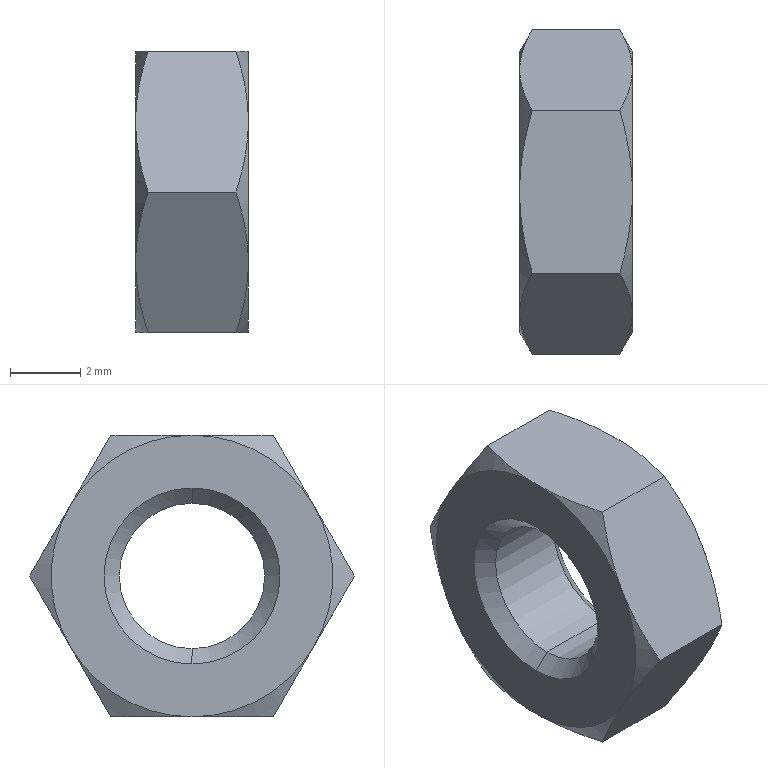Part | SolidWorks | features RefAxis 3, RevCut 2, 3DProfileFeature 1, Extrusion 1 | 1 solid | 26 faces | box 3.2 x 9.238 x 8 mm | volume 130.688 mm3 | cone 16 | plane 8 | cylinder 2 | commonest cylinder face diameters 4.134 x2
STEP:
#1=CARTESIAN_POINT('',(2.767,0.,2.067));
#2=VERTEX_POINT('',#1);
#3=CARTESIAN_POINT('',(2.767,0.,-2.067));
#4=VERTEX_POINT('',#3);
#5=CARTESIAN_POINT('',(2.767,0.,0.));
#6=DIRECTION('',(1.,0.,0.));
#7=DIRECTION('',(0.,0.,-1.));
#8=AXIS2_PLACEMENT_3D('',#5,#6,#7);
#9=CIRCLE('',#8,2.067);
#10=EDGE_CURVE('',#2,#4,#9,.T.);
#11=ORIENTED_EDGE('',*,*,#10,.F.);
#12=CARTESIAN_POINT('',(3.2,0.,2.5));
#13=VERTEX_POINT('',#12);
#14=CARTESIAN_POINT('',(3.2,0.,2.5));
#15=DIRECTION('',(0.7071,0.,0.7071));
#16=VECTOR('',#15,1000.);
#17=LINE('',#14,#16);
#18=EDGE_CURVE('',#2,#13,#17,.T.);
#19=ORIENTED_EDGE('',*,*,#18,.T.);
#20=CARTESIAN_POINT('',(3.2,0.,-2.5));
#21=VERTEX_POINT('',#20);
#22=CARTESIAN_POINT('',(3.2,0.,0.));
#23=DIRECTION('',(1.,0.,0.));
#24=DIRECTION('',(0.,0.,-1.));
#25=AXIS2_PLACEMENT_3D('',#22,#23,#24);
#26=CIRCLE('',#25,2.5);
#27=EDGE_CURVE('',#13,#21,#26,.T.);
#28=ORIENTED_EDGE('',*,*,#27,.T.);
#29=CARTESIAN_POINT('',(3.2,0.,-2.5));
#30=DIRECTION('',(0.7071,0.,-0.7071));
#31=VECTOR('',#30,1000.);
#32=LINE('',#29,#31);
#33=EDGE_CURVE('',#4,#21,#32,.T.);
#34=ORIENTED_EDGE('',*,*,#33,.F.);
#35=EDGE_LOOP('',(#11,#19,#28,#34));
#36=FACE_OUTER_BOUND('',#35,.T.);
#37=CARTESIAN_POINT('',(3.2,0.,0.));
#38=DIRECTION('',(1.,0.,0.));
#39=DIRECTION('',(0.,0.,-1.));
#40=AXIS2_PLACEMENT_3D('',#37,#38,#39);
#41=CONICAL_SURFACE('',#40,2.5,0.7854);
#42=ADVANCED_FACE('',(#36),#41,.F.);
#43=CARTESIAN_POINT('',(0.433,0.,2.067));
#44=VERTEX_POINT('',#43);
#45=CARTESIAN_POINT('',(0.433,0.,-2.067));
#46=VERTEX_POINT('',#45);
#47=CARTESIAN_POINT('',(0.433,0.,0.));
#48=DIRECTION('',(1.,0.,0.));
#49=DIRECTION('',(0.,0.,-1.));
#50=AXIS2_PLACEMENT_3D('',#47,#48,#49);
#51=CIRCLE('',#50,2.067);
#52=EDGE_CURVE('',#44,#46,#51,.T.);
#53=ORIENTED_EDGE('',*,*,#52,.F.);
#54=CARTESIAN_POINT('',(3.2,0.,2.067));
#55=DIRECTION('',(1.,0.,0.));
#56=VECTOR('',#55,1000.);
#57=LINE('',#54,#56);
#58=EDGE_CURVE('',#44,#2,#57,.T.);
#59=ORIENTED_EDGE('',*,*,#58,.T.);
#60=ORIENTED_EDGE('',*,*,#10,.T.);
#61=CARTESIAN_POINT('',(3.2,0.,-2.067));
#62=DIRECTION('',(1.,0.,0.));
#63=VECTOR('',#62,1000.);
#64=LINE('',#61,#63);
#65=EDGE_CURVE('',#46,#4,#64,.T.);
#66=ORIENTED_EDGE('',*,*,#65,.F.);
#67=EDGE_LOOP('',(#53,#59,#60,#66));
#68=FACE_OUTER_BOUND('',#67,.T.);
#69=CARTESIAN_POINT('',(3.2,0.,0.));
#70=DIRECTION('',(1.,0.,0.));
#71=DIRECTION('',(0.,0.,-1.));
#72=AXIS2_PLACEMENT_3D('',#69,#70,#71);
#73=CYLINDRICAL_SURFACE('',#72,2.067);
#74=ADVANCED_FACE('',(#68),#73,.F.);
#75=ORIENTED_EDGE('',*,*,#52,.T.);
#76=CARTESIAN_POINT('',(0.,0.,-2.5));
#77=VERTEX_POINT('',#76);
#78=CARTESIAN_POINT('',(0.433,0.,-2.067));
#79=DIRECTION('',(-0.7071,0.,-0.7071));
#80=VECTOR('',#79,1000.);
#81=LINE('',#78,#80);
#82=EDGE_CURVE('',#46,#77,#81,.T.);
#83=ORIENTED_EDGE('',*,*,#82,.T.);
#84=CARTESIAN_POINT('',(0.,0.,2.5));
#85=VERTEX_POINT('',#84);
#86=CARTESIAN_POINT('',(0.,0.,0.));
#87=DIRECTION('',(1.,0.,0.));
#88=DIRECTION('',(0.,0.,-1.));
#89=AXIS2_PLACEMENT_3D('',#86,#87,#88);
#90=CIRCLE('',#89,2.5);
#91=EDGE_CURVE('',#85,#77,#90,.T.);
#92=ORIENTED_EDGE('',*,*,#91,.F.);
#93=CARTESIAN_POINT('',(0.433,0.,2.067));
#94=DIRECTION('',(-0.7071,0.,0.7071));
#95=VECTOR('',#94,1000.);
#96=LINE('',#93,#95);
#97=EDGE_CURVE('',#44,#85,#96,.T.);
#98=ORIENTED_EDGE('',*,*,#97,.F.);
#99=EDGE_LOOP('',(#75,#83,#92,#98));
#100=FACE_OUTER_BOUND('',#99,.T.);
#101=CARTESIAN_POINT('',(0.433,0.,0.));
#102=DIRECTION('',(-1.,0.,0.));
#103=DIRECTION('',(0.,0.,1.));
#104=AXIS2_PLACEMENT_3D('',#101,#102,#103);
#105=CONICAL_SURFACE('',#104,2.067,0.7854);
#106=ADVANCED_FACE('',(#100),#105,.F.);
#107=ORIENTED_EDGE('',*,*,#91,.T.);
#108=CARTESIAN_POINT('',(0.,0.,0.));
#109=DIRECTION('',(1.,0.,0.));
#110=DIRECTION('',(0.,0.,-1.));
#111=AXIS2_PLACEMENT_3D('',#108,#109,#110);
#112=CIRCLE('',#111,2.5);
#113=EDGE_CURVE('',#77,#85,#112,.T.);
#114=ORIENTED_EDGE('',*,*,#113,.T.);
#115=EDGE_LOOP('',(#107,#114));
#116=FACE_BOUND('',#115,.T.);
#117=CARTESIAN_POINT('',(0.,0.,-4.));
#118=VERTEX_POINT('',#117);
#119=CARTESIAN_POINT('',(0.,3.464,-2.));
#120=VERTEX_POINT('',#119);
#121=CARTESIAN_POINT('',(0.,0.,0.));
#122=DIRECTION('',(1.,0.,0.));
#123=DIRECTION('',(0.,0.,-1.));
#124=AXIS2_PLACEMENT_3D('',#121,#122,#123);
#125=CIRCLE('',#124,4.);
#126=EDGE_CURVE('',#118,#120,#125,.T.);
#127=ORIENTED_EDGE('',*,*,#126,.F.);
#128=CARTESIAN_POINT('',(0.,-3.464,-2.));
#129=VERTEX_POINT('',#128);
#130=CARTESIAN_POINT('',(0.,0.,0.));
#131=DIRECTION('',(-1.,0.,0.));
#132=DIRECTION('',(0.,0.,-1.));
#133=AXIS2_PLACEMENT_3D('',#130,#131,#132);
#134=CIRCLE('',#133,4.);
#135=EDGE_CURVE('',#118,#129,#134,.T.);
#136=ORIENTED_EDGE('',*,*,#135,.T.);
#137=CARTESIAN_POINT('',(0.,-3.464,2.));
#138=VERTEX_POINT('',#137);
#139=CARTESIAN_POINT('',(0.,0.,0.));
#140=DIRECTION('',(-1.,0.,0.));
#141=DIRECTION('',(0.,0.,-1.));
#142=AXIS2_PLACEMENT_3D('',#139,#140,#141);
#143=CIRCLE('',#142,4.);
#144=EDGE_CURVE('',#129,#138,#143,.T.);
#145=ORIENTED_EDGE('',*,*,#144,.T.);
#146=CARTESIAN_POINT('',(0.,0.,4.));
#147=VERTEX_POINT('',#146);
#148=CARTESIAN_POINT('',(0.,0.,0.));
#149=DIRECTION('',(-1.,0.,0.));
#150=DIRECTION('',(0.,0.,-1.));
#151=AXIS2_PLACEMENT_3D('',#148,#149,#150);
#152=CIRCLE('',#151,4.);
#153=EDGE_CURVE('',#138,#147,#152,.T.);
#154=ORIENTED_EDGE('',*,*,#153,.T.);
#155=CARTESIAN_POINT('',(0.,3.464,2.));
#156=VERTEX_POINT('',#155);
#157=CARTESIAN_POINT('',(0.,0.,0.));
#158=DIRECTION('',(-1.,0.,0.));
#159=DIRECTION('',(0.,0.,-1.));
#160=AXIS2_PLACEMENT_3D('',#157,#158,#159);
#161=CIRCLE('',#160,4.);
#162=EDGE_CURVE('',#147,#156,#161,.T.);
#163=ORIENTED_EDGE('',*,*,#162,.T.);
#164=CARTESIAN_POINT('',(0.,0.,0.));
#165=DIRECTION('',(-1.,0.,0.));
#166=DIRECTION('',(0.,0.,-1.));
#167=AXIS2_PLACEMENT_3D('',#164,#165,#166);
#168=CIRCLE('',#167,4.);
#169=EDGE_CURVE('',#156,#120,#168,.T.);
#170=ORIENTED_EDGE('',*,*,#169,.T.);
#171=EDGE_LOOP('',(#127,#136,#145,#154,#163,#170));
#172=FACE_OUTER_BOUND('',#171,.T.);
#173=CARTESIAN_POINT('',(0.,2.309,4.));
#174=DIRECTION('',(1.,0.,0.));
#175=DIRECTION('',(0.,0.,-1.));
#176=AXIS2_PLACEMENT_3D('',#173,#174,#175);
#177=PLANE('',#176);
#178=ADVANCED_FACE('',(#116,#172),#177,.F.);
#179=ORIENTED_EDGE('',*,*,#126,.T.);
#180=CARTESIAN_POINT('',(0.3573,2.309,-4.));
#181=VERTEX_POINT('',#180);
#182=CARTESIAN_POINT('',(0.3573,2.309,-4.));
#183=CARTESIAN_POINT('',(0.1392,2.687,-3.346));
#184=CARTESIAN_POINT('',(0.,3.071,-2.681));
#185=CARTESIAN_POINT('',(0.,3.464,-2.));
#186=B_SPLINE_CURVE_WITH_KNOTS('',3,(#182,#183,#184,#185),.UNSPECIFIED.,.F.,.F.,(4,4),(0.000000238,0.002337),.UNSPECIFIED.);
#187=EDGE_CURVE('',#181,#120,#186,.T.);
#188=ORIENTED_EDGE('',*,*,#187,.F.);
#189=CARTESIAN_POINT('',(0.,0.,-4.));
#190=CARTESIAN_POINT('',(0.,0.3912,-4.));
#191=CARTESIAN_POINT('',(0.03459,0.7871,-4.));
#192=CARTESIAN_POINT('',(0.1597,1.558,-4.));
#193=CARTESIAN_POINT('',(0.2494,1.936,-4.));
#194=CARTESIAN_POINT('',(0.3573,2.309,-4.));
#195=B_SPLINE_CURVE_WITH_KNOTS('',3,(#189,#190,#191,#192,#193,#194),.UNSPECIFIED.,.F.,.F.,(4,2,4),(0.006652,0.007822,0.008992),.UNSPECIFIED.);
#196=EDGE_CURVE('',#118,#181,#195,.T.);
#197=ORIENTED_EDGE('',*,*,#196,.F.);
#198=EDGE_LOOP('',(#179,#188,#197));
#199=FACE_OUTER_BOUND('',#198,.T.);
#200=CARTESIAN_POINT('',(0.,0.,0.));
#201=DIRECTION('',(1.,0.,0.));
#202=DIRECTION('',(0.,0.,-1.));
#203=AXIS2_PLACEMENT_3D('',#200,#201,#202);
#204=CONICAL_SURFACE('',#203,4.,1.047);
#205=ADVANCED_FACE('',(#199),#204,.T.);
#206=CARTESIAN_POINT('',(0.3573,4.619,0.));
#207=VERTEX_POINT('',#206);
#208=CARTESIAN_POINT('',(0.,3.464,-2.));
#209=CARTESIAN_POINT('',(0.,3.66,-1.661));
#210=CARTESIAN_POINT('',(0.03421,3.856,-1.322));
#211=CARTESIAN_POINT('',(0.1587,4.24,-0.6554));
#212=CARTESIAN_POINT('',(0.2485,4.43,-0.3264));
#213=CARTESIAN_POINT('',(0.3573,4.619,0.));
#214=B_SPLINE_CURVE_WITH_KNOTS('',3,(#208,#209,#210,#211,#212,#213),.UNSPECIFIED.,.F.,.F.,(4,2,4),(0.002337,0.003501,0.004665),.UNSPECIFIED.);
#215=EDGE_CURVE('',#120,#207,#214,.T.);
#216=ORIENTED_EDGE('',*,*,#215,.F.);
#217=ORIENTED_EDGE('',*,*,#169,.F.);
#218=CARTESIAN_POINT('',(0.3573,4.619,0.));
#219=CARTESIAN_POINT('',(0.1392,4.241,0.6543));
#220=CARTESIAN_POINT('',(0.,3.858,1.319));
#221=CARTESIAN_POINT('',(0.,3.464,2.));
#222=B_SPLINE_CURVE_WITH_KNOTS('',3,(#218,#219,#220,#221),.UNSPECIFIED.,.F.,.F.,(4,4),(0.000000238,0.002337),.UNSPECIFIED.);
#223=EDGE_CURVE('',#207,#156,#222,.T.);
#224=ORIENTED_EDGE('',*,*,#223,.F.);
#225=EDGE_LOOP('',(#216,#217,#224));
#226=FACE_OUTER_BOUND('',#225,.T.);
#227=CARTESIAN_POINT('',(0.,0.,0.));
#228=DIRECTION('',(1.,0.,0.));
#229=DIRECTION('',(0.,0.,-1.));
#230=AXIS2_PLACEMENT_3D('',#227,#228,#229);
#231=CONICAL_SURFACE('',#230,4.,1.047);
#232=ADVANCED_FACE('',(#226),#231,.T.);
#233=ORIENTED_EDGE('',*,*,#162,.F.);
#234=CARTESIAN_POINT('',(0.3573,2.309,4.));
#235=VERTEX_POINT('',#234);
#236=CARTESIAN_POINT('',(0.3573,2.309,4.));
#237=CARTESIAN_POINT('',(0.2494,1.936,4.));
#238=CARTESIAN_POINT('',(0.1597,1.558,4.));
#239=CARTESIAN_POINT('',(0.03459,0.7871,4.));
#240=CARTESIAN_POINT('',(0.,0.3912,4.));
#241=CARTESIAN_POINT('',(0.,0.,4.));
#242=B_SPLINE_CURVE_WITH_KNOTS('',3,(#236,#237,#238,#239,#240,#241),.UNSPECIFIED.,.F.,.F.,(4,2,4),(0.01114,0.01231,0.01348),.UNSPECIFIED.);
#243=EDGE_CURVE('',#235,#147,#242,.T.);
#244=ORIENTED_EDGE('',*,*,#243,.F.);
#245=CARTESIAN_POINT('',(0.,3.464,2.));
#246=CARTESIAN_POINT('',(0.,3.268,2.339));
#247=CARTESIAN_POINT('',(0.03421,3.072,2.678));
#248=CARTESIAN_POINT('',(0.1587,2.688,3.345));
#249=CARTESIAN_POINT('',(0.2485,2.498,3.674));
#250=CARTESIAN_POINT('',(0.3573,2.309,4.));
#251=B_SPLINE_CURVE_WITH_KNOTS('',3,(#245,#246,#247,#248,#249,#250),.UNSPECIFIED.,.F.,.F.,(4,2,4),(0.002337,0.003501,0.004665),.UNSPECIFIED.);
#252=EDGE_CURVE('',#156,#235,#251,.T.);
#253=ORIENTED_EDGE('',*,*,#252,.F.);
#254=EDGE_LOOP('',(#233,#244,#253));
#255=FACE_OUTER_BOUND('',#254,.T.);
#256=CARTESIAN_POINT('',(0.,0.,0.));
#257=DIRECTION('',(1.,0.,0.));
#258=DIRECTION('',(0.,0.,-1.));
#259=AXIS2_PLACEMENT_3D('',#256,#257,#258);
#260=CONICAL_SURFACE('',#259,4.,1.047);
#261=ADVANCED_FACE('',(#255),#260,.T.);
#262=ORIENTED_EDGE('',*,*,#153,.F.);
#263=CARTESIAN_POINT('',(0.3573,-2.309,4.));
#264=VERTEX_POINT('',#263);
#265=CARTESIAN_POINT('',(0.3573,-2.309,4.));
#266=CARTESIAN_POINT('',(0.1392,-2.687,3.346));
#267=CARTESIAN_POINT('',(0.,-3.071,2.681));
#268=CARTESIAN_POINT('',(0.,-3.464,2.));
#269=B_SPLINE_CURVE_WITH_KNOTS('',3,(#265,#266,#267,#268),.UNSPECIFIED.,.F.,.F.,(4,4),(0.000000238,0.002337),.UNSPECIFIED.);
#270=EDGE_CURVE('',#264,#138,#269,.T.);
#271=ORIENTED_EDGE('',*,*,#270,.F.);
#272=CARTESIAN_POINT('',(0.,0.,4.));
#273=CARTESIAN_POINT('',(0.,-0.3908,4.));
#274=CARTESIAN_POINT('',(0.03364,-0.7786,4.));
#275=CARTESIAN_POINT('',(0.1579,-1.549,4.));
#276=CARTESIAN_POINT('',(0.2487,-1.933,4.));
#277=CARTESIAN_POINT('',(0.3573,-2.309,4.));
#278=B_SPLINE_CURVE_WITH_KNOTS('',3,(#272,#273,#274,#275,#276,#277),.UNSPECIFIED.,.F.,.F.,(4,2,4),(0.01348,0.01465,0.01582),.UNSPECIFIED.);
#279=EDGE_CURVE('',#147,#264,#278,.T.);
#280=ORIENTED_EDGE('',*,*,#279,.F.);
#281=EDGE_LOOP('',(#262,#271,#280));
#282=FACE_OUTER_BOUND('',#281,.T.);
#283=CARTESIAN_POINT('',(0.,0.,0.));
#284=DIRECTION('',(1.,0.,0.));
#285=DIRECTION('',(0.,0.,-1.));
#286=AXIS2_PLACEMENT_3D('',#283,#284,#285);
#287=CONICAL_SURFACE('',#286,4.,1.047);
#288=ADVANCED_FACE('',(#282),#287,.T.);
#289=ORIENTED_EDGE('',*,*,#144,.F.);
#290=CARTESIAN_POINT('',(0.3573,-4.619,0.));
#291=VERTEX_POINT('',#290);
#292=CARTESIAN_POINT('',(0.3573,-4.619,0.));
#293=CARTESIAN_POINT('',(0.1392,-4.241,-0.6543));
#294=CARTESIAN_POINT('',(0.,-3.858,-1.319));
#295=CARTESIAN_POINT('',(0.,-3.464,-2.));
#296=B_SPLINE_CURVE_WITH_KNOTS('',3,(#292,#293,#294,#295),.UNSPECIFIED.,.F.,.F.,(4,4),(0.000000238,0.002337),.UNSPECIFIED.);
#297=EDGE_CURVE('',#291,#129,#296,.T.);
#298=ORIENTED_EDGE('',*,*,#297,.F.);
#299=CARTESIAN_POINT('',(0.,-3.464,2.));
#300=CARTESIAN_POINT('',(0.,-3.66,1.661));
#301=CARTESIAN_POINT('',(0.03421,-3.856,1.322));
#302=CARTESIAN_POINT('',(0.1587,-4.24,0.6554));
#303=CARTESIAN_POINT('',(0.2485,-4.43,0.3264));
#304=CARTESIAN_POINT('',(0.3573,-4.619,0.));
#305=B_SPLINE_CURVE_WITH_KNOTS('',3,(#299,#300,#301,#302,#303,#304),.UNSPECIFIED.,.F.,.F.,(4,2,4),(0.002337,0.003501,0.004665),.UNSPECIFIED.);
#306=EDGE_CURVE('',#138,#291,#305,.T.);
#307=ORIENTED_EDGE('',*,*,#306,.F.);
#308=EDGE_LOOP('',(#289,#298,#307));
#309=FACE_OUTER_BOUND('',#308,.T.);
#310=CARTESIAN_POINT('',(0.,0.,0.));
#311=DIRECTION('',(1.,0.,0.));
#312=DIRECTION('',(0.,0.,-1.));
#313=AXIS2_PLACEMENT_3D('',#310,#311,#312);
#314=CONICAL_SURFACE('',#313,4.,1.047);
#315=ADVANCED_FACE('',(#309),#314,.T.);
#316=ORIENTED_EDGE('',*,*,#135,.F.);
#317=CARTESIAN_POINT('',(0.3573,-2.309,-4.));
#318=VERTEX_POINT('',#317);
#319=CARTESIAN_POINT('',(0.3573,-2.309,-4.));
#320=CARTESIAN_POINT('',(0.2487,-1.933,-4.));
#321=CARTESIAN_POINT('',(0.1579,-1.549,-4.));
#322=CARTESIAN_POINT('',(0.03364,-0.7786,-4.));
#323=CARTESIAN_POINT('',(0.,-0.3908,-4.));
#324=CARTESIAN_POINT('',(0.,0.,-4.));
#325=B_SPLINE_CURVE_WITH_KNOTS('',3,(#319,#320,#321,#322,#323,#324),.UNSPECIFIED.,.F.,.F.,(4,2,4),(0.004314,0.005483,0.006652),.UNSPECIFIED.);
#326=EDGE_CURVE('',#318,#118,#325,.T.);
#327=ORIENTED_EDGE('',*,*,#326,.F.);
#328=CARTESIAN_POINT('',(0.,-3.464,-2.));
#329=CARTESIAN_POINT('',(0.,-3.268,-2.339));
#330=CARTESIAN_POINT('',(0.03421,-3.072,-2.678));
#331=CARTESIAN_POINT('',(0.1587,-2.688,-3.345));
#332=CARTESIAN_POINT('',(0.2485,-2.498,-3.674));
#333=CARTESIAN_POINT('',(0.3573,-2.309,-4.));
#334=B_SPLINE_CURVE_WITH_KNOTS('',3,(#328,#329,#330,#331,#332,#333),.UNSPECIFIED.,.F.,.F.,(4,2,4),(0.002337,0.003501,0.004665),.UNSPECIFIED.);
#335=EDGE_CURVE('',#129,#318,#334,.T.);
#336=ORIENTED_EDGE('',*,*,#335,.F.);
#337=EDGE_LOOP('',(#316,#327,#336));
#338=FACE_OUTER_BOUND('',#337,.T.);
#339=CARTESIAN_POINT('',(0.,0.,0.));
#340=DIRECTION('',(1.,0.,0.));
#341=DIRECTION('',(0.,0.,-1.));
#342=AXIS2_PLACEMENT_3D('',#339,#340,#341);
#343=CONICAL_SURFACE('',#342,4.,1.047);
#344=ADVANCED_FACE('',(#338),#343,.T.);
#345=CARTESIAN_POINT('',(2.843,2.309,4.));
#346=VERTEX_POINT('',#345);
#347=CARTESIAN_POINT('',(3.2,2.309,4.));
#348=DIRECTION('',(-1.,0.,0.));
#349=VECTOR('',#348,1000.);
#350=LINE('',#347,#349);
#351=EDGE_CURVE('',#346,#235,#350,.T.);
#352=ORIENTED_EDGE('',*,*,#351,.F.);
#353=CARTESIAN_POINT('',(3.2,3.464,2.));
#354=VERTEX_POINT('',#353);
#355=CARTESIAN_POINT('',(2.843,2.309,4.));
#356=CARTESIAN_POINT('',(3.061,2.687,3.346));
#357=CARTESIAN_POINT('',(3.2,3.071,2.681));
#358=CARTESIAN_POINT('',(3.2,3.464,2.));
#359=B_SPLINE_CURVE_WITH_KNOTS('',3,(#355,#356,#357,#358),.UNSPECIFIED.,.F.,.F.,(4,4),(0.000000238,0.002337),.UNSPECIFIED.);
#360=EDGE_CURVE('',#346,#354,#359,.T.);
#361=ORIENTED_EDGE('',*,*,#360,.T.);
#362=CARTESIAN_POINT('',(2.843,4.619,0.));
#363=VERTEX_POINT('',#362);
#364=CARTESIAN_POINT('',(3.2,3.464,2.));
#365=CARTESIAN_POINT('',(3.2,3.66,1.661));
#366=CARTESIAN_POINT('',(3.166,3.856,1.322));
#367=CARTESIAN_POINT('',(3.041,4.24,0.6554));
#368=CARTESIAN_POINT('',(2.952,4.43,0.3264));
#369=CARTESIAN_POINT('',(2.843,4.619,0.));
#370=B_SPLINE_CURVE_WITH_KNOTS('',3,(#364,#365,#366,#367,#368,#369),.UNSPECIFIED.,.F.,.F.,(4,2,4),(0.002337,0.003501,0.004665),.UNSPECIFIED.);
#371=EDGE_CURVE('',#354,#363,#370,.T.);
#372=ORIENTED_EDGE('',*,*,#371,.T.);
#373=CARTESIAN_POINT('',(3.2,4.619,0.));
#374=DIRECTION('',(-1.,0.,0.));
#375=VECTOR('',#374,1000.);
#376=LINE('',#373,#375);
#377=EDGE_CURVE('',#363,#207,#376,.T.);
#378=ORIENTED_EDGE('',*,*,#377,.T.);
#379=ORIENTED_EDGE('',*,*,#223,.T.);
#380=ORIENTED_EDGE('',*,*,#252,.T.);
#381=EDGE_LOOP('',(#352,#361,#372,#378,#379,#380));
#382=FACE_OUTER_BOUND('',#381,.T.);
#383=CARTESIAN_POINT('',(3.2,4.619,0.));
#384=DIRECTION('',(0.,-0.866,-0.5));
#385=DIRECTION('',(0.,0.5,-0.866));
#386=AXIS2_PLACEMENT_3D('',#383,#384,#385);
#387=PLANE('',#386);
#388=ADVANCED_FACE('',(#382),#387,.F.);
#389=CARTESIAN_POINT('',(2.843,-2.309,4.));
#390=VERTEX_POINT('',#389);
#391=CARTESIAN_POINT('',(3.2,-2.309,4.));
#392=DIRECTION('',(-1.,0.,0.));
#393=VECTOR('',#392,1000.);
#394=LINE('',#391,#393);
#395=EDGE_CURVE('',#390,#264,#394,.T.);
#396=ORIENTED_EDGE('',*,*,#395,.F.);
#397=CARTESIAN_POINT('',(3.2,0.,4.));
#398=VERTEX_POINT('',#397);
#399=CARTESIAN_POINT('',(2.843,-2.309,4.));
#400=CARTESIAN_POINT('',(2.951,-1.933,4.));
#401=CARTESIAN_POINT('',(3.042,-1.549,4.));
#402=CARTESIAN_POINT('',(3.166,-0.7786,4.));
#403=CARTESIAN_POINT('',(3.2,-0.3908,4.));
#404=CARTESIAN_POINT('',(3.2,0.,4.));
#405=B_SPLINE_CURVE_WITH_KNOTS('',3,(#399,#400,#401,#402,#403,#404),.UNSPECIFIED.,.F.,.F.,(4,2,4),(0.004314,0.005483,0.006652),.UNSPECIFIED.);
#406=EDGE_CURVE('',#390,#398,#405,.T.);
#407=ORIENTED_EDGE('',*,*,#406,.T.);
#408=CARTESIAN_POINT('',(3.2,0.,4.));
#409=CARTESIAN_POINT('',(3.2,0.3912,4.));
#410=CARTESIAN_POINT('',(3.165,0.7871,4.));
#411=CARTESIAN_POINT('',(3.04,1.558,4.));
#412=CARTESIAN_POINT('',(2.951,1.936,4.));
#413=CARTESIAN_POINT('',(2.843,2.309,4.));
#414=B_SPLINE_CURVE_WITH_KNOTS('',3,(#408,#409,#410,#411,#412,#413),.UNSPECIFIED.,.F.,.F.,(4,2,4),(0.006652,0.007822,0.008992),.UNSPECIFIED.);
#415=EDGE_CURVE('',#398,#346,#414,.T.);
#416=ORIENTED_EDGE('',*,*,#415,.T.);
#417=ORIENTED_EDGE('',*,*,#351,.T.);
#418=ORIENTED_EDGE('',*,*,#243,.T.);
#419=ORIENTED_EDGE('',*,*,#279,.T.);
#420=EDGE_LOOP('',(#396,#407,#416,#417,#418,#419));
#421=FACE_OUTER_BOUND('',#420,.T.);
#422=CARTESIAN_POINT('',(3.2,2.309,4.));
#423=DIRECTION('',(0.,0.,-1.));
#424=DIRECTION('',(-1.,0.,0.));
#425=AXIS2_PLACEMENT_3D('',#422,#423,#424);
#426=PLANE('',#425);
#427=ADVANCED_FACE('',(#421),#426,.F.);
#428=CARTESIAN_POINT('',(2.843,-4.619,0.));
#429=VERTEX_POINT('',#428);
#430=CARTESIAN_POINT('',(3.2,-4.619,0.));
#431=DIRECTION('',(-1.,0.,0.));
#432=VECTOR('',#431,1000.);
#433=LINE('',#430,#432);
#434=EDGE_CURVE('',#429,#291,#433,.T.);
#435=ORIENTED_EDGE('',*,*,#434,.F.);
#436=CARTESIAN_POINT('',(3.2,-3.464,2.));
#437=VERTEX_POINT('',#436);
#438=CARTESIAN_POINT('',(2.843,-4.619,0.));
#439=CARTESIAN_POINT('',(3.061,-4.241,0.6543));
#440=CARTESIAN_POINT('',(3.2,-3.858,1.319));
#441=CARTESIAN_POINT('',(3.2,-3.464,2.));
#442=B_SPLINE_CURVE_WITH_KNOTS('',3,(#438,#439,#440,#441),.UNSPECIFIED.,.F.,.F.,(4,4),(0.000000238,0.002337),.UNSPECIFIED.);
#443=EDGE_CURVE('',#429,#437,#442,.T.);
#444=ORIENTED_EDGE('',*,*,#443,.T.);
#445=CARTESIAN_POINT('',(3.2,-3.464,2.));
#446=CARTESIAN_POINT('',(3.2,-3.268,2.339));
#447=CARTESIAN_POINT('',(3.166,-3.072,2.678));
#448=CARTESIAN_POINT('',(3.041,-2.688,3.345));
#449=CARTESIAN_POINT('',(2.952,-2.498,3.674));
#450=CARTESIAN_POINT('',(2.843,-2.309,4.));
#451=B_SPLINE_CURVE_WITH_KNOTS('',3,(#445,#446,#447,#448,#449,#450),.UNSPECIFIED.,.F.,.F.,(4,2,4),(0.002337,0.003501,0.004665),.UNSPECIFIED.);
#452=EDGE_CURVE('',#437,#390,#451,.T.);
#453=ORIENTED_EDGE('',*,*,#452,.T.);
#454=ORIENTED_EDGE('',*,*,#395,.T.);
#455=ORIENTED_EDGE('',*,*,#270,.T.);
#456=ORIENTED_EDGE('',*,*,#306,.T.);
#457=EDGE_LOOP('',(#435,#444,#453,#454,#455,#456));
#458=FACE_OUTER_BOUND('',#457,.T.);
#459=CARTESIAN_POINT('',(3.2,-2.309,4.));
#460=DIRECTION('',(0.,0.866,-0.5));
#461=DIRECTION('',(0.,0.5,0.866));
#462=AXIS2_PLACEMENT_3D('',#459,#460,#461);
#463=PLANE('',#462);
#464=ADVANCED_FACE('',(#458),#463,.F.);
#465=CARTESIAN_POINT('',(2.843,-2.309,-4.));
#466=VERTEX_POINT('',#465);
#467=CARTESIAN_POINT('',(3.2,-2.309,-4.));
#468=DIRECTION('',(-1.,0.,0.));
#469=VECTOR('',#468,1000.);
#470=LINE('',#467,#469);
#471=EDGE_CURVE('',#466,#318,#470,.T.);
#472=ORIENTED_EDGE('',*,*,#471,.F.);
#473=CARTESIAN_POINT('',(3.2,-3.464,-2.));
#474=VERTEX_POINT('',#473);
#475=CARTESIAN_POINT('',(2.843,-2.309,-4.));
#476=CARTESIAN_POINT('',(3.061,-2.687,-3.346));
#477=CARTESIAN_POINT('',(3.2,-3.071,-2.681));
#478=CARTESIAN_POINT('',(3.2,-3.464,-2.));
#479=B_SPLINE_CURVE_WITH_KNOTS('',3,(#475,#476,#477,#478),.UNSPECIFIED.,.F.,.F.,(4,4),(0.000000238,0.002337),.UNSPECIFIED.);
#480=EDGE_CURVE('',#466,#474,#479,.T.);
#481=ORIENTED_EDGE('',*,*,#480,.T.);
#482=CARTESIAN_POINT('',(3.2,-3.464,-2.));
#483=CARTESIAN_POINT('',(3.2,-3.66,-1.661));
#484=CARTESIAN_POINT('',(3.166,-3.856,-1.322));
#485=CARTESIAN_POINT('',(3.041,-4.24,-0.6554));
#486=CARTESIAN_POINT('',(2.952,-4.43,-0.3264));
#487=CARTESIAN_POINT('',(2.843,-4.619,0.));
#488=B_SPLINE_CURVE_WITH_KNOTS('',3,(#482,#483,#484,#485,#486,#487),.UNSPECIFIED.,.F.,.F.,(4,2,4),(0.002337,0.003501,0.004665),.UNSPECIFIED.);
#489=EDGE_CURVE('',#474,#429,#488,.T.);
#490=ORIENTED_EDGE('',*,*,#489,.T.);
#491=ORIENTED_EDGE('',*,*,#434,.T.);
#492=ORIENTED_EDGE('',*,*,#297,.T.);
#493=ORIENTED_EDGE('',*,*,#335,.T.);
#494=EDGE_LOOP('',(#472,#481,#490,#491,#492,#493));
#495=FACE_OUTER_BOUND('',#494,.T.);
#496=CARTESIAN_POINT('',(3.2,-4.619,0.));
#497=DIRECTION('',(0.,0.866,0.5));
#498=DIRECTION('',(0.,-0.5,0.866));
#499=AXIS2_PLACEMENT_3D('',#496,#497,#498);
#500=PLANE('',#499);
#501=ADVANCED_FACE('',(#495),#500,.F.);
#502=CARTESIAN_POINT('',(2.843,2.309,-4.));
#503=VERTEX_POINT('',#502);
#504=CARTESIAN_POINT('',(3.2,2.309,-4.));
#505=DIRECTION('',(-1.,0.,0.));
#506=VECTOR('',#505,1000.);
#507=LINE('',#504,#506);
#508=EDGE_CURVE('',#503,#181,#507,.T.);
#509=ORIENTED_EDGE('',*,*,#508,.F.);
#510=CARTESIAN_POINT('',(3.2,0.,-4.));
#511=VERTEX_POINT('',#510);
#512=CARTESIAN_POINT('',(2.843,2.309,-4.));
#513=CARTESIAN_POINT('',(2.951,1.936,-4.));
#514=CARTESIAN_POINT('',(3.04,1.558,-4.));
#515=CARTESIAN_POINT('',(3.165,0.7871,-4.));
#516=CARTESIAN_POINT('',(3.2,0.3912,-4.));
#517=CARTESIAN_POINT('',(3.2,0.,-4.));
#518=B_SPLINE_CURVE_WITH_KNOTS('',3,(#512,#513,#514,#515,#516,#517),.UNSPECIFIED.,.F.,.F.,(4,2,4),(0.01114,0.01231,0.01348),.UNSPECIFIED.);
#519=EDGE_CURVE('',#503,#511,#518,.T.);
#520=ORIENTED_EDGE('',*,*,#519,.T.);
#521=CARTESIAN_POINT('',(3.2,0.,-4.));
#522=CARTESIAN_POINT('',(3.2,-0.3908,-4.));
#523=CARTESIAN_POINT('',(3.166,-0.7786,-4.));
#524=CARTESIAN_POINT('',(3.042,-1.549,-4.));
#525=CARTESIAN_POINT('',(2.951,-1.933,-4.));
#526=CARTESIAN_POINT('',(2.843,-2.309,-4.));
#527=B_SPLINE_CURVE_WITH_KNOTS('',3,(#521,#522,#523,#524,#525,#526),.UNSPECIFIED.,.F.,.F.,(4,2,4),(0.01348,0.01465,0.01582),.UNSPECIFIED.);
#528=EDGE_CURVE('',#511,#466,#527,.T.);
#529=ORIENTED_EDGE('',*,*,#528,.T.);
#530=ORIENTED_EDGE('',*,*,#471,.T.);
#531=ORIENTED_EDGE('',*,*,#326,.T.);
#532=ORIENTED_EDGE('',*,*,#196,.T.);
#533=EDGE_LOOP('',(#509,#520,#529,#530,#531,#532));
#534=FACE_OUTER_BOUND('',#533,.T.);
#535=CARTESIAN_POINT('',(3.2,-2.309,-4.));
#536=DIRECTION('',(0.,0.,1.));
#537=DIRECTION('',(1.,0.,0.));
#538=AXIS2_PLACEMENT_3D('',#535,#536,#537);
#539=PLANE('',#538);
#540=ADVANCED_FACE('',(#534),#539,.F.);
#541=ORIENTED_EDGE('',*,*,#377,.F.);
#542=CARTESIAN_POINT('',(3.2,3.464,-2.));
#543=VERTEX_POINT('',#542);
#544=CARTESIAN_POINT('',(2.843,4.619,0.));
#545=CARTESIAN_POINT('',(3.061,4.241,-0.6543));
#546=CARTESIAN_POINT('',(3.2,3.858,-1.319));
#547=CARTESIAN_POINT('',(3.2,3.464,-2.));
#548=B_SPLINE_CURVE_WITH_KNOTS('',3,(#544,#545,#546,#547),.UNSPECIFIED.,.F.,.F.,(4,4),(0.000000238,0.002337),.UNSPECIFIED.);
#549=EDGE_CURVE('',#363,#543,#548,.T.);
#550=ORIENTED_EDGE('',*,*,#549,.T.);
#551=CARTESIAN_POINT('',(3.2,3.464,-2.));
#552=CARTESIAN_POINT('',(3.2,3.268,-2.339));
#553=CARTESIAN_POINT('',(3.166,3.072,-2.678));
#554=CARTESIAN_POINT('',(3.041,2.688,-3.345));
#555=CARTESIAN_POINT('',(2.952,2.498,-3.674));
#556=CARTESIAN_POINT('',(2.843,2.309,-4.));
#557=B_SPLINE_CURVE_WITH_KNOTS('',3,(#551,#552,#553,#554,#555,#556),.UNSPECIFIED.,.F.,.F.,(4,2,4),(0.002337,0.003501,0.004665),.UNSPECIFIED.);
#558=EDGE_CURVE('',#543,#503,#557,.T.);
#559=ORIENTED_EDGE('',*,*,#558,.T.);
#560=ORIENTED_EDGE('',*,*,#508,.T.);
#561=ORIENTED_EDGE('',*,*,#187,.T.);
#562=ORIENTED_EDGE('',*,*,#215,.T.);
#563=EDGE_LOOP('',(#541,#550,#559,#560,#561,#562));
#564=FACE_OUTER_BOUND('',#563,.T.);
#565=CARTESIAN_POINT('',(3.2,2.309,-4.));
#566=DIRECTION('',(0.,-0.866,0.5));
#567=DIRECTION('',(0.,-0.5,-0.866));
#568=AXIS2_PLACEMENT_3D('',#565,#566,#567);
#569=PLANE('',#568);
#570=ADVANCED_FACE('',(#564),#569,.F.);
#571=ORIENTED_EDGE('',*,*,#558,.F.);
#572=CARTESIAN_POINT('',(3.2,0.,0.));
#573=DIRECTION('',(1.,0.,0.));
#574=DIRECTION('',(0.,0.,-1.));
#575=AXIS2_PLACEMENT_3D('',#572,#573,#574);
#576=CIRCLE('',#575,4.);
#577=EDGE_CURVE('',#511,#543,#576,.T.);
#578=ORIENTED_EDGE('',*,*,#577,.F.);
#579=ORIENTED_EDGE('',*,*,#519,.F.);
#580=EDGE_LOOP('',(#571,#578,#579));
#581=FACE_OUTER_BOUND('',#580,.T.);
#582=CARTESIAN_POINT('',(1.6,0.,0.));
#583=DIRECTION('',(-1.,0.,0.));
#584=DIRECTION('',(0.,0.,1.));
#585=AXIS2_PLACEMENT_3D('',#582,#583,#584);
#586=CONICAL_SURFACE('',#585,6.771,1.047);
#587=ADVANCED_FACE('',(#581),#586,.T.);
#588=CARTESIAN_POINT('',(3.2,0.,0.));
#589=DIRECTION('',(-1.,0.,0.));
#590=DIRECTION('',(0.,0.,-1.));
#591=AXIS2_PLACEMENT_3D('',#588,#589,#590);
#592=CIRCLE('',#591,4.);
#593=EDGE_CURVE('',#354,#543,#592,.T.);
#594=ORIENTED_EDGE('',*,*,#593,.T.);
#595=ORIENTED_EDGE('',*,*,#549,.F.);
#596=ORIENTED_EDGE('',*,*,#371,.F.);
#597=EDGE_LOOP('',(#594,#595,#596));
#598=FACE_OUTER_BOUND('',#597,.T.);
#599=CARTESIAN_POINT('',(1.6,0.,0.));
#600=DIRECTION('',(-1.,0.,0.));
#601=DIRECTION('',(0.,0.,1.));
#602=AXIS2_PLACEMENT_3D('',#599,#600,#601);
#603=CONICAL_SURFACE('',#602,6.771,1.047);
#604=ADVANCED_FACE('',(#598),#603,.T.);
#605=CARTESIAN_POINT('',(3.2,0.,0.));
#606=DIRECTION('',(-1.,0.,0.));
#607=DIRECTION('',(0.,0.,-1.));
#608=AXIS2_PLACEMENT_3D('',#605,#606,#607);
#609=CIRCLE('',#608,4.);
#610=EDGE_CURVE('',#398,#354,#609,.T.);
#611=ORIENTED_EDGE('',*,*,#610,.T.);
#612=ORIENTED_EDGE('',*,*,#360,.F.);
#613=ORIENTED_EDGE('',*,*,#415,.F.);
#614=EDGE_LOOP('',(#611,#612,#613));
#615=FACE_OUTER_BOUND('',#614,.T.);
#616=CARTESIAN_POINT('',(1.6,0.,0.));
#617=DIRECTION('',(-1.,0.,0.));
#618=DIRECTION('',(0.,0.,1.));
#619=AXIS2_PLACEMENT_3D('',#616,#617,#618);
#620=CONICAL_SURFACE('',#619,6.771,1.047);
#621=ADVANCED_FACE('',(#615),#620,.T.);
#622=CARTESIAN_POINT('',(3.2,0.,0.));
#623=DIRECTION('',(-1.,0.,0.));
#624=DIRECTION('',(0.,0.,-1.));
#625=AXIS2_PLACEMENT_3D('',#622,#623,#624);
#626=CIRCLE('',#625,4.);
#627=EDGE_CURVE('',#437,#398,#626,.T.);
#628=ORIENTED_EDGE('',*,*,#627,.T.);
#629=ORIENTED_EDGE('',*,*,#406,.F.);
#630=ORIENTED_EDGE('',*,*,#452,.F.);
#631=EDGE_LOOP('',(#628,#629,#630));
#632=FACE_OUTER_BOUND('',#631,.T.);
#633=CARTESIAN_POINT('',(1.6,0.,0.));
#634=DIRECTION('',(-1.,0.,0.));
#635=DIRECTION('',(0.,0.,1.));
#636=AXIS2_PLACEMENT_3D('',#633,#634,#635);
#637=CONICAL_SURFACE('',#636,6.771,1.047);
#638=ADVANCED_FACE('',(#632),#637,.T.);
#639=ORIENTED_EDGE('',*,*,#489,.F.);
#640=CARTESIAN_POINT('',(3.2,0.,0.));
#641=DIRECTION('',(-1.,0.,0.));
#642=DIRECTION('',(0.,0.,-1.));
#643=AXIS2_PLACEMENT_3D('',#640,#641,#642);
#644=CIRCLE('',#643,4.);
#645=EDGE_CURVE('',#474,#437,#644,.T.);
#646=ORIENTED_EDGE('',*,*,#645,.T.);
#647=ORIENTED_EDGE('',*,*,#443,.F.);
#648=EDGE_LOOP('',(#639,#646,#647));
#649=FACE_OUTER_BOUND('',#648,.T.);
#650=CARTESIAN_POINT('',(1.6,0.,0.));
#651=DIRECTION('',(-1.,0.,0.));
#652=DIRECTION('',(0.,0.,1.));
#653=AXIS2_PLACEMENT_3D('',#650,#651,#652);
#654=CONICAL_SURFACE('',#653,6.771,1.047);
#655=ADVANCED_FACE('',(#649),#654,.T.);
#656=ORIENTED_EDGE('',*,*,#528,.F.);
#657=CARTESIAN_POINT('',(3.2,0.,0.));
#658=DIRECTION('',(-1.,0.,0.));
#659=DIRECTION('',(0.,0.,-1.));
#660=AXIS2_PLACEMENT_3D('',#657,#658,#659);
#661=CIRCLE('',#660,4.);
#662=EDGE_CURVE('',#511,#474,#661,.T.);
#663=ORIENTED_EDGE('',*,*,#662,.T.);
#664=ORIENTED_EDGE('',*,*,#480,.F.);
#665=EDGE_LOOP('',(#656,#663,#664));
#666=FACE_OUTER_BOUND('',#665,.T.);
#667=CARTESIAN_POINT('',(1.6,0.,0.));
#668=DIRECTION('',(-1.,0.,0.));
#669=DIRECTION('',(0.,0.,1.));
#670=AXIS2_PLACEMENT_3D('',#667,#668,#669);
#671=CONICAL_SURFACE('',#670,6.771,1.047);
#672=ADVANCED_FACE('',(#666),#671,.T.);
#673=CARTESIAN_POINT('',(3.2,0.,0.));
#674=DIRECTION('',(1.,0.,0.));
#675=DIRECTION('',(0.,0.,-1.));
#676=AXIS2_PLACEMENT_3D('',#673,#674,#675);
#677=CIRCLE('',#676,2.5);
#678=EDGE_CURVE('',#21,#13,#677,.T.);
#679=ORIENTED_EDGE('',*,*,#678,.F.);
#680=ORIENTED_EDGE('',*,*,#27,.F.);
#681=EDGE_LOOP('',(#679,#680));
#682=FACE_BOUND('',#681,.T.);
#683=ORIENTED_EDGE('',*,*,#662,.F.);
#684=ORIENTED_EDGE('',*,*,#577,.T.);
#685=ORIENTED_EDGE('',*,*,#593,.F.);
#686=ORIENTED_EDGE('',*,*,#610,.F.);
#687=ORIENTED_EDGE('',*,*,#627,.F.);
#688=ORIENTED_EDGE('',*,*,#645,.F.);
#689=EDGE_LOOP('',(#683,#684,#685,#686,#687,#688));
#690=FACE_OUTER_BOUND('',#689,.T.);
#691=CARTESIAN_POINT('',(3.2,2.309,4.));
#692=DIRECTION('',(1.,0.,0.));
#693=DIRECTION('',(0.,0.,-1.));
#694=AXIS2_PLACEMENT_3D('',#691,#692,#693);
#695=PLANE('',#694);
#696=ADVANCED_FACE('',(#682,#690),#695,.T.);
#697=ORIENTED_EDGE('',*,*,#82,.F.);
#698=CARTESIAN_POINT('',(0.433,0.,0.));
#699=DIRECTION('',(1.,0.,0.));
#700=DIRECTION('',(0.,0.,-1.));
#701=AXIS2_PLACEMENT_3D('',#698,#699,#700);
#702=CIRCLE('',#701,2.067);
#703=EDGE_CURVE('',#46,#44,#702,.T.);
#704=ORIENTED_EDGE('',*,*,#703,.T.);
#705=ORIENTED_EDGE('',*,*,#97,.T.);
#706=ORIENTED_EDGE('',*,*,#113,.F.);
#707=EDGE_LOOP('',(#697,#704,#705,#706));
#708=FACE_OUTER_BOUND('',#707,.T.);
#709=CARTESIAN_POINT('',(0.433,0.,0.));
#710=DIRECTION('',(-1.,0.,0.));
#711=DIRECTION('',(0.,0.,1.));
#712=AXIS2_PLACEMENT_3D('',#709,#710,#711);
#713=CONICAL_SURFACE('',#712,2.067,0.7854);
#714=ADVANCED_FACE('',(#708),#713,.F.);
#715=ORIENTED_EDGE('',*,*,#58,.F.);
#716=ORIENTED_EDGE('',*,*,#703,.F.);
#717=ORIENTED_EDGE('',*,*,#65,.T.);
#718=CARTESIAN_POINT('',(2.767,0.,0.));
#719=DIRECTION('',(1.,0.,0.));
#720=DIRECTION('',(0.,0.,-1.));
#721=AXIS2_PLACEMENT_3D('',#718,#719,#720);
#722=CIRCLE('',#721,2.067);
#723=EDGE_CURVE('',#4,#2,#722,.T.);
#724=ORIENTED_EDGE('',*,*,#723,.T.);
#725=EDGE_LOOP('',(#715,#716,#717,#724));
#726=FACE_OUTER_BOUND('',#725,.T.);
#727=CARTESIAN_POINT('',(3.2,0.,0.));
#728=DIRECTION('',(1.,0.,0.));
#729=DIRECTION('',(0.,0.,-1.));
#730=AXIS2_PLACEMENT_3D('',#727,#728,#729);
#731=CYLINDRICAL_SURFACE('',#730,2.067);
#732=ADVANCED_FACE('',(#726),#731,.F.);
#733=ORIENTED_EDGE('',*,*,#18,.F.);
#734=ORIENTED_EDGE('',*,*,#723,.F.);
#735=ORIENTED_EDGE('',*,*,#33,.T.);
#736=ORIENTED_EDGE('',*,*,#678,.T.);
#737=EDGE_LOOP('',(#733,#734,#735,#736));
#738=FACE_OUTER_BOUND('',#737,.T.);
#739=CARTESIAN_POINT('',(3.2,0.,0.));
#740=DIRECTION('',(1.,0.,0.));
#741=DIRECTION('',(0.,0.,-1.));
#742=AXIS2_PLACEMENT_3D('',#739,#740,#741);
#743=CONICAL_SURFACE('',#742,2.5,0.7854);
#744=ADVANCED_FACE('',(#738),#743,.F.);
#745=CLOSED_SHELL('',(#42,#74,#106,#178,#205,#232,#261,#288,#315,#344,#388,#427,#464,#501,#540,#570,#587,#604,#621,#638,#655,#672,#696,#714,#732,#744));
#746=MANIFOLD_SOLID_BREP('',#745);
#747=CARTESIAN_POINT('',(0.,0.,0.));
#748=DIRECTION('',(0.,0.,1.));
#749=DIRECTION('',(1.,0.,0.));
#750=AXIS2_PLACEMENT_3D('',#747,#748,#749);
#751=(LENGTH_UNIT()NAMED_UNIT(*)SI_UNIT(.MILLI.,.METRE.));
#752=UNCERTAINTY_MEASURE_WITH_UNIT(LENGTH_MEASURE(0.00001),#751,'','');
#753=(NAMED_UNIT(*)PLANE_ANGLE_UNIT()SI_UNIT($,.RADIAN.));
#754=(NAMED_UNIT(*)SI_UNIT($,.STERADIAN.)SOLID_ANGLE_UNIT());
#755=(GEOMETRIC_REPRESENTATION_CONTEXT(3)GLOBAL_UNCERTAINTY_ASSIGNED_CONTEXT((#752))GLOBAL_UNIT_ASSIGNED_CONTEXT((#751,#753,#754))REPRESENTATION_CONTEXT('',''));
#756=ADVANCED_BREP_SHAPE_REPRESENTATION('',(#746,#750),#755);